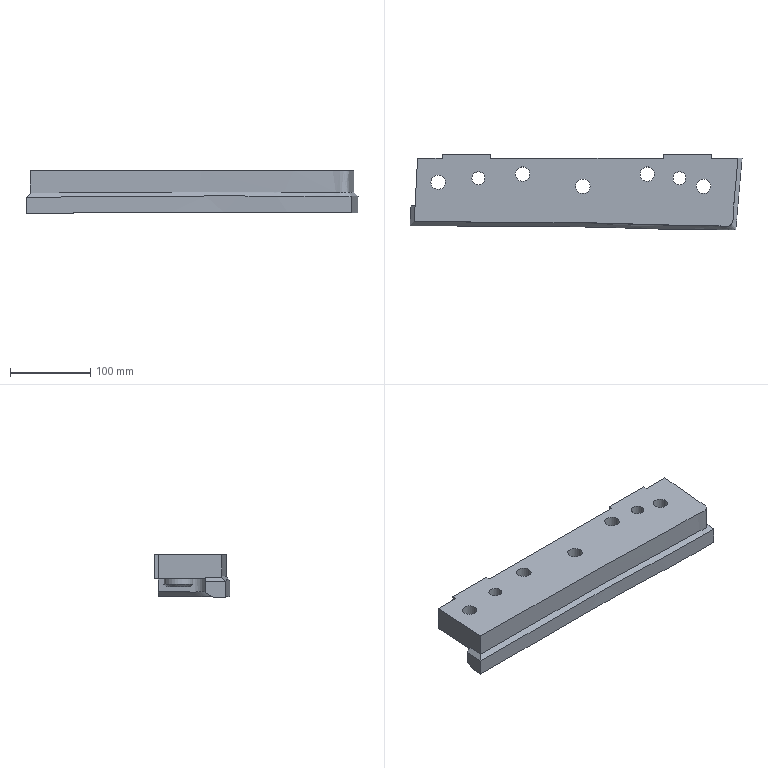Part | NX | features solid 2 | 1 solid | 44 faces | box 412.786 x 94.233 x 53.058 mm | volume 1150670 mm3 | plane 22 | cylinder 14 | spline 6 | cone 2 | commonest cylinder face diameters 18 x5 26 x5 16 x2 36 x2